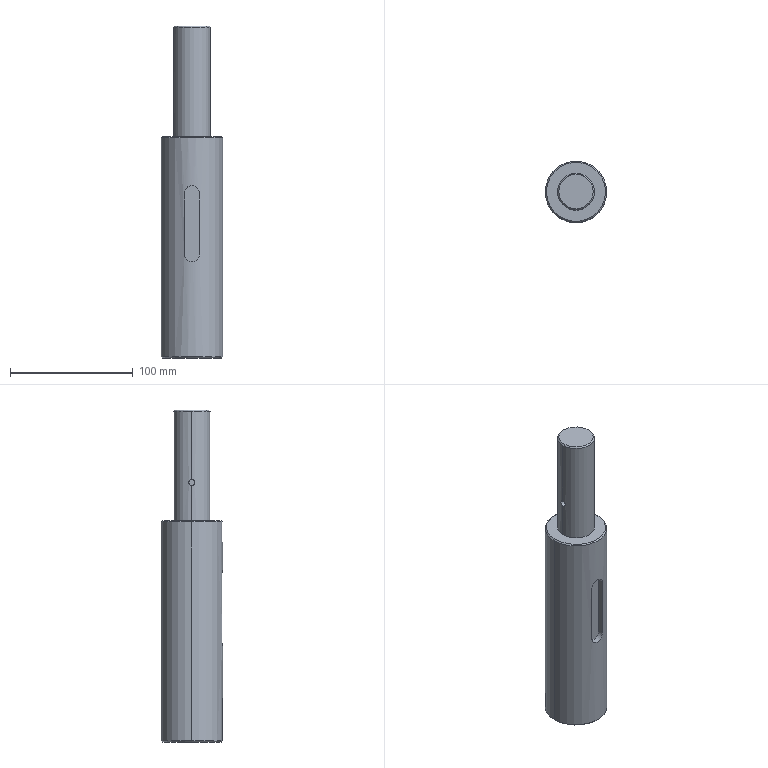Part | SolidWorks | features ICE 3, Chamfer 1, Extrusion 1 | 1 solid | 22 faces | box 50 x 50 x 270 mm | volume 413348 mm3 | cylinder 9 | plane 7 | cone 6 | commonest cylinder face diameters 12 x3 5 x2 30 x2 50 x2
STEP:
#1=CARTESIAN_POINT('',(-15.,0.,213.5));
#2=VERTEX_POINT('',#1);
#3=CARTESIAN_POINT('',(-15.,0.,208.5));
#4=VERTEX_POINT('',#3);
#5=CARTESIAN_POINT('',(-15.,0.,213.5));
#6=CARTESIAN_POINT('',(-15.,-0.1655,213.5));
#7=CARTESIAN_POINT('',(-14.997,-0.3282,213.484));
#8=CARTESIAN_POINT('',(-14.987,-0.6481,213.42));
#9=CARTESIAN_POINT('',(-14.979,-0.8071,213.372));
#10=CARTESIAN_POINT('',(-14.96,-1.11,213.246));
#11=CARTESIAN_POINT('',(-14.948,-1.253,213.169));
#12=CARTESIAN_POINT('',(-14.923,-1.525,212.988));
#13=CARTESIAN_POINT('',(-14.909,-1.653,212.882));
#14=CARTESIAN_POINT('',(-14.868,-1.998,212.537));
#15=CARTESIAN_POINT('',(-14.841,-2.184,212.259));
#16=CARTESIAN_POINT('',(-14.811,-2.372,211.808));
#17=CARTESIAN_POINT('',(-14.804,-2.42,211.65));
#18=CARTESIAN_POINT('',(-14.793,-2.484,211.327));
#19=CARTESIAN_POINT('',(-14.79,-2.5,211.164));
#20=CARTESIAN_POINT('',(-14.79,-2.5,210.838));
#21=CARTESIAN_POINT('',(-14.793,-2.484,210.672));
#22=CARTESIAN_POINT('',(-14.804,-2.42,210.351));
#23=CARTESIAN_POINT('',(-14.811,-2.372,210.195));
#24=CARTESIAN_POINT('',(-14.831,-2.247,209.892));
#25=CARTESIAN_POINT('',(-14.843,-2.169,209.746));
#26=CARTESIAN_POINT('',(-14.868,-1.988,209.475));
#27=CARTESIAN_POINT('',(-14.882,-1.884,209.349));
#28=CARTESIAN_POINT('',(-14.909,-1.651,209.116));
#29=CARTESIAN_POINT('',(-14.923,-1.525,209.013));
#30=CARTESIAN_POINT('',(-14.948,-1.255,208.832));
#31=CARTESIAN_POINT('',(-14.96,-1.109,208.753));
#32=CARTESIAN_POINT('',(-14.979,-0.8061,208.628));
#33=CARTESIAN_POINT('',(-14.987,-0.6502,208.58));
#34=CARTESIAN_POINT('',(-14.997,-0.3292,208.516));
#35=CARTESIAN_POINT('',(-15.,-0.1633,208.5));
#36=CARTESIAN_POINT('',(-15.,0.,208.5));
#37=B_SPLINE_CURVE_WITH_KNOTS('',3,(#5,#6,#7,#8,#9,#10,#11,#12,#13,#14,#15,#16,#17,#18,#19,#20,#21,#22,#23,#24,#25,#26,#27,#28,#29,#30,#31,#32,#33,#34,#35,#36),.UNSPECIFIED.,.F.,.F.,(4,2,2,2,2,2,2,2,2,2,2,2,2,2,2,4),(0.,0.0004894,0.0009787,0.001468,0.001957,0.002936,0.003426,0.003915,0.004404,0.004894,0.005383,0.005872,0.006362,0.006851,0.00734,0.00783),.UNSPECIFIED.);
#38=EDGE_CURVE('',#2,#4,#37,.T.);
#39=ORIENTED_EDGE('',*,*,#38,.F.);
#40=CARTESIAN_POINT('',(-10.,0.,213.5));
#41=VERTEX_POINT('',#40);
#42=CARTESIAN_POINT('',(-20.,0.,213.5));
#43=DIRECTION('',(1.,0.,0.));
#44=VECTOR('',#43,1000.);
#45=LINE('',#42,#44);
#46=EDGE_CURVE('',#2,#41,#45,.T.);
#47=ORIENTED_EDGE('',*,*,#46,.T.);
#48=CARTESIAN_POINT('',(-10.,0.,208.5));
#49=VERTEX_POINT('',#48);
#50=CARTESIAN_POINT('',(-10.,0.,211.));
#51=DIRECTION('',(1.,0.,0.));
#52=DIRECTION('',(0.,0.,-1.));
#53=AXIS2_PLACEMENT_3D('',#50,#51,#52);
#54=CIRCLE('',#53,2.5);
#55=EDGE_CURVE('',#41,#49,#54,.T.);
#56=ORIENTED_EDGE('',*,*,#55,.T.);
#57=CARTESIAN_POINT('',(-20.,0.,208.5));
#58=DIRECTION('',(1.,0.,0.));
#59=VECTOR('',#58,1000.);
#60=LINE('',#57,#59);
#61=EDGE_CURVE('',#4,#49,#60,.T.);
#62=ORIENTED_EDGE('',*,*,#61,.F.);
#63=EDGE_LOOP('',(#39,#47,#56,#62));
#64=FACE_OUTER_BOUND('',#63,.T.);
#65=CARTESIAN_POINT('',(-20.,0.,211.));
#66=DIRECTION('',(1.,0.,0.));
#67=DIRECTION('',(0.,0.,-1.));
#68=AXIS2_PLACEMENT_3D('',#65,#66,#67);
#69=CYLINDRICAL_SURFACE('',#68,2.5);
#70=ADVANCED_FACE('',(#64),#69,.F.);
#71=CARTESIAN_POINT('',(-24.,0.,0.));
#72=VERTEX_POINT('',#71);
#73=CARTESIAN_POINT('',(24.,0.,0.));
#74=VERTEX_POINT('',#73);
#75=CARTESIAN_POINT('',(0.,0.,0.));
#76=DIRECTION('',(0.,0.,-1.));
#77=DIRECTION('',(1.,0.,0.));
#78=AXIS2_PLACEMENT_3D('',#75,#76,#77);
#79=CIRCLE('',#78,24.);
#80=EDGE_CURVE('',#72,#74,#79,.T.);
#81=ORIENTED_EDGE('',*,*,#80,.F.);
#82=CARTESIAN_POINT('',(-25.,0.,1.));
#83=VERTEX_POINT('',#82);
#84=CARTESIAN_POINT('',(-25.,0.,1.));
#85=DIRECTION('',(-0.7071,0.,0.7071));
#86=VECTOR('',#85,1000.);
#87=LINE('',#84,#86);
#88=EDGE_CURVE('',#72,#83,#87,.T.);
#89=ORIENTED_EDGE('',*,*,#88,.T.);
#90=CARTESIAN_POINT('',(25.,0.,1.));
#91=VERTEX_POINT('',#90);
#92=CARTESIAN_POINT('',(0.,0.,1.));
#93=DIRECTION('',(0.,0.,1.));
#94=DIRECTION('',(1.,0.,0.));
#95=AXIS2_PLACEMENT_3D('',#92,#93,#94);
#96=CIRCLE('',#95,25.);
#97=EDGE_CURVE('',#91,#83,#96,.T.);
#98=ORIENTED_EDGE('',*,*,#97,.F.);
#99=CARTESIAN_POINT('',(25.,0.,1.));
#100=DIRECTION('',(0.7071,0.,0.7071));
#101=VECTOR('',#100,1000.);
#102=LINE('',#99,#101);
#103=EDGE_CURVE('',#74,#91,#102,.T.);
#104=ORIENTED_EDGE('',*,*,#103,.F.);
#105=EDGE_LOOP('',(#81,#89,#98,#104));
#106=FACE_OUTER_BOUND('',#105,.T.);
#107=CARTESIAN_POINT('',(0.,0.,1.));
#108=DIRECTION('',(0.,0.,1.));
#109=DIRECTION('',(1.,0.,0.));
#110=AXIS2_PLACEMENT_3D('',#107,#108,#109);
#111=CONICAL_SURFACE('',#110,25.,0.7854);
#112=ADVANCED_FACE('',(#106),#111,.T.);
#113=CARTESIAN_POINT('',(14.,0.,270.));
#114=VERTEX_POINT('',#113);
#115=CARTESIAN_POINT('',(-14.,0.,270.));
#116=VERTEX_POINT('',#115);
#117=CARTESIAN_POINT('',(0.,0.,270.));
#118=DIRECTION('',(0.,0.,1.));
#119=DIRECTION('',(1.,0.,0.));
#120=AXIS2_PLACEMENT_3D('',#117,#118,#119);
#121=CIRCLE('',#120,14.);
#122=EDGE_CURVE('',#114,#116,#121,.T.);
#123=ORIENTED_EDGE('',*,*,#122,.F.);
#124=CARTESIAN_POINT('',(15.,0.,269.));
#125=VERTEX_POINT('',#124);
#126=CARTESIAN_POINT('',(14.,0.,270.));
#127=DIRECTION('',(0.7071,0.,-0.7071));
#128=VECTOR('',#127,1000.);
#129=LINE('',#126,#128);
#130=EDGE_CURVE('',#114,#125,#129,.T.);
#131=ORIENTED_EDGE('',*,*,#130,.T.);
#132=CARTESIAN_POINT('',(-15.,0.,269.));
#133=VERTEX_POINT('',#132);
#134=CARTESIAN_POINT('',(0.,0.,269.));
#135=DIRECTION('',(0.,0.,-1.));
#136=DIRECTION('',(1.,0.,0.));
#137=AXIS2_PLACEMENT_3D('',#134,#135,#136);
#138=CIRCLE('',#137,15.);
#139=EDGE_CURVE('',#133,#125,#138,.T.);
#140=ORIENTED_EDGE('',*,*,#139,.F.);
#141=CARTESIAN_POINT('',(-14.,0.,270.));
#142=DIRECTION('',(-0.7071,0.,-0.7071));
#143=VECTOR('',#142,1000.);
#144=LINE('',#141,#143);
#145=EDGE_CURVE('',#116,#133,#144,.T.);
#146=ORIENTED_EDGE('',*,*,#145,.F.);
#147=EDGE_LOOP('',(#123,#131,#140,#146));
#148=FACE_OUTER_BOUND('',#147,.T.);
#149=CARTESIAN_POINT('',(0.,0.,270.));
#150=DIRECTION('',(0.,0.,-1.));
#151=DIRECTION('',(-1.,0.,0.));
#152=AXIS2_PLACEMENT_3D('',#149,#150,#151);
#153=CONICAL_SURFACE('',#152,14.,0.7854);
#154=ADVANCED_FACE('',(#148),#153,.T.);
#155=CARTESIAN_POINT('',(24.,0.,180.));
#156=VERTEX_POINT('',#155);
#157=CARTESIAN_POINT('',(-24.,0.,180.));
#158=VERTEX_POINT('',#157);
#159=CARTESIAN_POINT('',(0.,0.,180.));
#160=DIRECTION('',(0.,0.,1.));
#161=DIRECTION('',(1.,0.,0.));
#162=AXIS2_PLACEMENT_3D('',#159,#160,#161);
#163=CIRCLE('',#162,24.);
#164=EDGE_CURVE('',#156,#158,#163,.T.);
#165=ORIENTED_EDGE('',*,*,#164,.F.);
#166=CARTESIAN_POINT('',(25.,0.,179.));
#167=VERTEX_POINT('',#166);
#168=CARTESIAN_POINT('',(24.,0.,180.));
#169=DIRECTION('',(0.7071,0.,-0.7071));
#170=VECTOR('',#169,1000.);
#171=LINE('',#168,#170);
#172=EDGE_CURVE('',#156,#167,#171,.T.);
#173=ORIENTED_EDGE('',*,*,#172,.T.);
#174=CARTESIAN_POINT('',(-25.,0.,179.));
#175=VERTEX_POINT('',#174);
#176=CARTESIAN_POINT('',(0.,0.,179.));
#177=DIRECTION('',(0.,0.,-1.));
#178=DIRECTION('',(1.,0.,0.));
#179=AXIS2_PLACEMENT_3D('',#176,#177,#178);
#180=CIRCLE('',#179,25.);
#181=EDGE_CURVE('',#175,#167,#180,.T.);
#182=ORIENTED_EDGE('',*,*,#181,.F.);
#183=CARTESIAN_POINT('',(-24.,0.,180.));
#184=DIRECTION('',(-0.7071,0.,-0.7071));
#185=VECTOR('',#184,1000.);
#186=LINE('',#183,#185);
#187=EDGE_CURVE('',#158,#175,#186,.T.);
#188=ORIENTED_EDGE('',*,*,#187,.F.);
#189=EDGE_LOOP('',(#165,#173,#182,#188));
#190=FACE_OUTER_BOUND('',#189,.T.);
#191=CARTESIAN_POINT('',(0.,0.,180.));
#192=DIRECTION('',(0.,0.,-1.));
#193=DIRECTION('',(-1.,0.,0.));
#194=AXIS2_PLACEMENT_3D('',#191,#192,#193);
#195=CONICAL_SURFACE('',#194,24.,0.7854);
#196=ADVANCED_FACE('',(#190),#195,.T.);
#197=CARTESIAN_POINT('',(0.,-25.,140.23));
#198=VERTEX_POINT('',#197);
#199=CARTESIAN_POINT('',(6.,-24.269,134.23));
#200=VERTEX_POINT('',#199);
#201=CARTESIAN_POINT('',(0.,-25.,140.23));
#202=CARTESIAN_POINT('',(0.3927,-25.,140.23));
#203=CARTESIAN_POINT('',(0.7916,-24.99,140.19));
#204=CARTESIAN_POINT('',(1.562,-24.954,140.036));
#205=CARTESIAN_POINT('',(1.936,-24.928,139.923));
#206=CARTESIAN_POINT('',(2.482,-24.877,139.696));
#207=CARTESIAN_POINT('',(2.661,-24.859,139.611));
#208=CARTESIAN_POINT('',(3.007,-24.819,139.426));
#209=CARTESIAN_POINT('',(3.174,-24.798,139.325));
#210=CARTESIAN_POINT('',(3.498,-24.755,139.108));
#211=CARTESIAN_POINT('',(3.655,-24.732,138.992));
#212=CARTESIAN_POINT('',(3.957,-24.685,138.744));
#213=CARTESIAN_POINT('',(4.104,-24.661,138.612));
#214=CARTESIAN_POINT('',(4.521,-24.59,138.195));
#215=CARTESIAN_POINT('',(4.768,-24.542,137.894));
#216=CARTESIAN_POINT('',(5.202,-24.454,137.246));
#217=CARTESIAN_POINT('',(5.39,-24.413,136.895));
#218=CARTESIAN_POINT('',(5.691,-24.344,136.171));
#219=CARTESIAN_POINT('',(5.805,-24.317,135.797));
#220=CARTESIAN_POINT('',(5.96,-24.279,135.026));
#221=CARTESIAN_POINT('',(6.,-24.269,134.628));
#222=CARTESIAN_POINT('',(6.,-24.269,134.23));
#223=B_SPLINE_CURVE_WITH_KNOTS('',3,(#201,#202,#203,#204,#205,#206,#207,#208,#209,#210,#211,#212,#213,#214,#215,#216,#217,#218,#219,#220,#221,#222),.UNSPECIFIED.,.F.,.F.,(4,2,2,2,2,2,2,2,2,2,4),(0.009416,0.01059,0.01177,0.01236,0.01294,0.01353,0.01412,0.01529,0.01647,0.01765,0.01882),.UNSPECIFIED.);
#224=EDGE_CURVE('',#198,#200,#223,.T.);
#225=ORIENTED_EDGE('',*,*,#224,.F.);
#226=CARTESIAN_POINT('',(0.,-20.,140.23));
#227=VERTEX_POINT('',#226);
#228=CARTESIAN_POINT('',(0.,-140.,140.23));
#229=DIRECTION('',(0.,1.,0.));
#230=VECTOR('',#229,1000.);
#231=LINE('',#228,#230);
#232=EDGE_CURVE('',#198,#227,#231,.T.);
#233=ORIENTED_EDGE('',*,*,#232,.T.);
#234=CARTESIAN_POINT('',(6.,-20.,134.23));
#235=VERTEX_POINT('',#234);
#236=CARTESIAN_POINT('',(0.,-20.,134.23));
#237=DIRECTION('',(0.,1.,0.));
#238=DIRECTION('',(0.,0.,1.));
#239=AXIS2_PLACEMENT_3D('',#236,#237,#238);
#240=CIRCLE('',#239,6.);
#241=EDGE_CURVE('',#227,#235,#240,.T.);
#242=ORIENTED_EDGE('',*,*,#241,.T.);
#243=CARTESIAN_POINT('',(6.,-140.,134.23));
#244=DIRECTION('',(0.,1.,0.));
#245=VECTOR('',#244,1000.);
#246=LINE('',#243,#245);
#247=EDGE_CURVE('',#200,#235,#246,.T.);
#248=ORIENTED_EDGE('',*,*,#247,.F.);
#249=EDGE_LOOP('',(#225,#233,#242,#248));
#250=FACE_OUTER_BOUND('',#249,.T.);
#251=CARTESIAN_POINT('',(0.,-140.,134.23));
#252=DIRECTION('',(0.,1.,0.));
#253=DIRECTION('',(0.,0.,1.));
#254=AXIS2_PLACEMENT_3D('',#251,#252,#253);
#255=CYLINDRICAL_SURFACE('',#254,6.);
#256=ADVANCED_FACE('',(#250),#255,.F.);
#257=ORIENTED_EDGE('',*,*,#139,.T.);
#258=CARTESIAN_POINT('',(15.,0.,180.));
#259=VERTEX_POINT('',#258);
#260=CARTESIAN_POINT('',(15.,0.,270.));
#261=DIRECTION('',(0.,0.,-1.));
#262=VECTOR('',#261,1000.);
#263=LINE('',#260,#262);
#264=EDGE_CURVE('',#125,#259,#263,.T.);
#265=ORIENTED_EDGE('',*,*,#264,.T.);
#266=CARTESIAN_POINT('',(-15.,0.,180.));
#267=VERTEX_POINT('',#266);
#268=CARTESIAN_POINT('',(0.,0.,180.));
#269=DIRECTION('',(0.,0.,1.));
#270=DIRECTION('',(1.,0.,0.));
#271=AXIS2_PLACEMENT_3D('',#268,#269,#270);
#272=CIRCLE('',#271,15.);
#273=EDGE_CURVE('',#259,#267,#272,.T.);
#274=ORIENTED_EDGE('',*,*,#273,.T.);
#275=CARTESIAN_POINT('',(-15.,0.,270.));
#276=DIRECTION('',(0.,0.,-1.));
#277=VECTOR('',#276,1000.);
#278=LINE('',#275,#277);
#279=EDGE_CURVE('',#4,#267,#278,.T.);
#280=ORIENTED_EDGE('',*,*,#279,.F.);
#281=CARTESIAN_POINT('',(-15.,0.,208.5));
#282=CARTESIAN_POINT('',(-15.,0.3265,208.5));
#283=CARTESIAN_POINT('',(-14.989,0.656,208.566));
#284=CARTESIAN_POINT('',(-14.96,1.107,208.753));
#285=CARTESIAN_POINT('',(-14.948,1.253,208.831));
#286=CARTESIAN_POINT('',(-14.923,1.526,209.013));
#287=CARTESIAN_POINT('',(-14.909,1.651,209.116));
#288=CARTESIAN_POINT('',(-14.882,1.882,209.346));
#289=CARTESIAN_POINT('',(-14.868,1.987,209.475));
#290=CARTESIAN_POINT('',(-14.843,2.169,209.746));
#291=CARTESIAN_POINT('',(-14.831,2.246,209.889));
#292=CARTESIAN_POINT('',(-14.811,2.371,210.192));
#293=CARTESIAN_POINT('',(-14.804,2.42,210.35));
#294=CARTESIAN_POINT('',(-14.793,2.483,210.67));
#295=CARTESIAN_POINT('',(-14.79,2.5,210.833));
#296=CARTESIAN_POINT('',(-14.79,2.5,211.164));
#297=CARTESIAN_POINT('',(-14.793,2.484,211.326));
#298=CARTESIAN_POINT('',(-14.803,2.421,211.646));
#299=CARTESIAN_POINT('',(-14.811,2.372,211.805));
#300=CARTESIAN_POINT('',(-14.831,2.247,212.108));
#301=CARTESIAN_POINT('',(-14.842,2.17,212.251));
#302=CARTESIAN_POINT('',(-14.868,1.989,212.523));
#303=CARTESIAN_POINT('',(-14.882,1.884,212.651));
#304=CARTESIAN_POINT('',(-14.923,1.539,212.997));
#305=CARTESIAN_POINT('',(-14.95,1.261,213.183));
#306=CARTESIAN_POINT('',(-14.979,0.8099,213.371));
#307=CARTESIAN_POINT('',(-14.987,0.6518,213.419));
#308=CARTESIAN_POINT('',(-14.997,0.3289,213.484));
#309=CARTESIAN_POINT('',(-15.,0.1655,213.5));
#310=CARTESIAN_POINT('',(-15.,0.,213.5));
#311=B_SPLINE_CURVE_WITH_KNOTS('',3,(#281,#282,#283,#284,#285,#286,#287,#288,#289,#290,#291,#292,#293,#294,#295,#296,#297,#298,#299,#300,#301,#302,#303,#304,#305,#306,#307,#308,#309,#310),.UNSPECIFIED.,.F.,.F.,(4,2,2,2,2,2,2,2,2,2,2,2,2,2,4),(0.00783,0.008808,0.009298,0.009787,0.01028,0.01077,0.01125,0.01174,0.01223,0.01272,0.01321,0.0137,0.01468,0.01517,0.01566),.UNSPECIFIED.);
#312=EDGE_CURVE('',#4,#2,#311,.T.);
#313=ORIENTED_EDGE('',*,*,#312,.T.);
#314=CARTESIAN_POINT('',(-15.,0.,270.));
#315=DIRECTION('',(0.,0.,-1.));
#316=VECTOR('',#315,1000.);
#317=LINE('',#314,#316);
#318=EDGE_CURVE('',#133,#2,#317,.T.);
#319=ORIENTED_EDGE('',*,*,#318,.F.);
#320=EDGE_LOOP('',(#257,#265,#274,#280,#313,#319));
#321=FACE_OUTER_BOUND('',#320,.T.);
#322=CARTESIAN_POINT('',(0.,0.,270.));
#323=DIRECTION('',(0.,0.,-1.));
#324=DIRECTION('',(-1.,0.,0.));
#325=AXIS2_PLACEMENT_3D('',#322,#323,#324);
#326=CYLINDRICAL_SURFACE('',#325,15.);
#327=ADVANCED_FACE('',(#321),#326,.T.);
#328=ORIENTED_EDGE('',*,*,#181,.T.);
#329=CARTESIAN_POINT('',(25.,0.,180.));
#330=DIRECTION('',(0.,0.,-1.));
#331=VECTOR('',#330,1000.);
#332=LINE('',#329,#331);
#333=EDGE_CURVE('',#167,#91,#332,.T.);
#334=ORIENTED_EDGE('',*,*,#333,.T.);
#335=ORIENTED_EDGE('',*,*,#97,.T.);
#336=CARTESIAN_POINT('',(-25.,0.,180.));
#337=DIRECTION('',(0.,0.,-1.));
#338=VECTOR('',#337,1000.);
#339=LINE('',#336,#338);
#340=EDGE_CURVE('',#175,#83,#339,.T.);
#341=ORIENTED_EDGE('',*,*,#340,.F.);
#342=EDGE_LOOP('',(#328,#334,#335,#341));
#343=FACE_OUTER_BOUND('',#342,.T.);
#344=CARTESIAN_POINT('',(0.,0.,180.));
#345=DIRECTION('',(0.,0.,-1.));
#346=DIRECTION('',(-1.,0.,0.));
#347=AXIS2_PLACEMENT_3D('',#344,#345,#346);
#348=CYLINDRICAL_SURFACE('',#347,25.);
#349=ADVANCED_FACE('',(#343),#348,.T.);
#350=ORIENTED_EDGE('',*,*,#333,.F.);
#351=CARTESIAN_POINT('',(0.,0.,179.));
#352=DIRECTION('',(0.,0.,-1.));
#353=DIRECTION('',(1.,0.,0.));
#354=AXIS2_PLACEMENT_3D('',#351,#352,#353);
#355=CIRCLE('',#354,25.);
#356=EDGE_CURVE('',#167,#175,#355,.T.);
#357=ORIENTED_EDGE('',*,*,#356,.T.);
#358=ORIENTED_EDGE('',*,*,#340,.T.);
#359=CARTESIAN_POINT('',(0.,0.,1.));
#360=DIRECTION('',(0.,0.,1.));
#361=DIRECTION('',(1.,0.,0.));
#362=AXIS2_PLACEMENT_3D('',#359,#360,#361);
#363=CIRCLE('',#362,25.);
#364=EDGE_CURVE('',#83,#91,#363,.T.);
#365=ORIENTED_EDGE('',*,*,#364,.T.);
#366=EDGE_LOOP('',(#350,#357,#358,#365));
#367=FACE_OUTER_BOUND('',#366,.T.);
#368=CARTESIAN_POINT('',(6.,-24.269,84.23));
#369=VERTEX_POINT('',#368);
#370=CARTESIAN_POINT('',(6.,-24.269,180.));
#371=DIRECTION('',(0.,0.,-1.));
#372=VECTOR('',#371,1000.);
#373=LINE('',#370,#372);
#374=EDGE_CURVE('',#200,#369,#373,.T.);
#375=ORIENTED_EDGE('',*,*,#374,.T.);
#376=CARTESIAN_POINT('',(-6.,-24.269,84.23));
#377=VERTEX_POINT('',#376);
#378=CARTESIAN_POINT('',(6.,-24.269,84.23));
#379=CARTESIAN_POINT('',(6.,-24.269,83.832));
#380=CARTESIAN_POINT('',(5.961,-24.279,83.441));
#381=CARTESIAN_POINT('',(5.846,-24.307,82.865));
#382=CARTESIAN_POINT('',(5.798,-24.318,82.674));
#383=CARTESIAN_POINT('',(5.683,-24.345,82.297));
#384=CARTESIAN_POINT('',(5.616,-24.361,82.109));
#385=CARTESIAN_POINT('',(5.39,-24.413,81.565));
#386=CARTESIAN_POINT('',(5.206,-24.453,81.221));
#387=CARTESIAN_POINT('',(4.771,-24.542,80.57));
#388=CARTESIAN_POINT('',(4.518,-24.59,80.263));
#389=CARTESIAN_POINT('',(3.967,-24.685,79.712));
#390=CARTESIAN_POINT('',(3.666,-24.732,79.464));
#391=CARTESIAN_POINT('',(3.011,-24.82,79.025));
#392=CARTESIAN_POINT('',(2.664,-24.86,78.84));
#393=CARTESIAN_POINT('',(2.123,-24.91,78.615));
#394=CARTESIAN_POINT('',(1.939,-24.925,78.548));
#395=CARTESIAN_POINT('',(1.563,-24.952,78.434));
#396=CARTESIAN_POINT('',(1.37,-24.963,78.385));
#397=CARTESIAN_POINT('',(0.7883,-24.991,78.269));
#398=CARTESIAN_POINT('',(0.3981,-25.,78.23));
#399=CARTESIAN_POINT('',(-0.3876,-25.,78.23));
#400=CARTESIAN_POINT('',(-0.7868,-24.991,78.269));
#401=CARTESIAN_POINT('',(-1.557,-24.954,78.422));
#402=CARTESIAN_POINT('',(-1.932,-24.928,78.536));
#403=CARTESIAN_POINT('',(-2.478,-24.878,78.762));
#404=CARTESIAN_POINT('',(-2.658,-24.859,78.847));
#405=CARTESIAN_POINT('',(-3.004,-24.819,79.032));
#406=CARTESIAN_POINT('',(-3.172,-24.799,79.133));
#407=CARTESIAN_POINT('',(-3.658,-24.733,79.458));
#408=CARTESIAN_POINT('',(-3.963,-24.686,79.707));
#409=CARTESIAN_POINT('',(-4.519,-24.59,80.263));
#410=CARTESIAN_POINT('',(-4.766,-24.542,80.565));
#411=CARTESIAN_POINT('',(-5.201,-24.454,81.213));
#412=CARTESIAN_POINT('',(-5.389,-24.413,81.564));
#413=CARTESIAN_POINT('',(-5.691,-24.344,82.288));
#414=CARTESIAN_POINT('',(-5.805,-24.317,82.662));
#415=CARTESIAN_POINT('',(-5.96,-24.279,83.434));
#416=CARTESIAN_POINT('',(-6.,-24.269,83.832));
#417=CARTESIAN_POINT('',(-6.,-24.269,84.23));
#418=B_SPLINE_CURVE_WITH_KNOTS('',3,(#378,#379,#380,#381,#382,#383,#384,#385,#386,#387,#388,#389,#390,#391,#392,#393,#394,#395,#396,#397,#398,#399,#400,#401,#402,#403,#404,#405,#406,#407,#408,#409,#410,#411,#412,#413,#414,#415,#416,#417),.UNSPECIFIED.,.F.,.F.,(4,2,2,2,2,2,2,2,2,2,2,2,2,2,2,2,2,2,2,4),(0.,0.001176,0.001765,0.002353,0.003529,0.004705,0.005882,0.007058,0.007646,0.008235,0.009411,0.01059,0.01176,0.01235,0.01294,0.01412,0.01529,0.01647,0.01765,0.01882),.UNSPECIFIED.);
#419=EDGE_CURVE('',#369,#377,#418,.T.);
#420=ORIENTED_EDGE('',*,*,#419,.T.);
#421=CARTESIAN_POINT('',(-6.,-24.269,134.23));
#422=VERTEX_POINT('',#421);
#423=CARTESIAN_POINT('',(-6.,-24.269,180.));
#424=DIRECTION('',(0.,0.,1.));
#425=VECTOR('',#424,1000.);
#426=LINE('',#423,#425);
#427=EDGE_CURVE('',#377,#422,#426,.T.);
#428=ORIENTED_EDGE('',*,*,#427,.T.);
#429=CARTESIAN_POINT('',(-6.,-24.269,134.23));
#430=CARTESIAN_POINT('',(-6.,-24.269,134.628));
#431=CARTESIAN_POINT('',(-5.961,-24.279,135.019));
#432=CARTESIAN_POINT('',(-5.846,-24.307,135.596));
#433=CARTESIAN_POINT('',(-5.798,-24.318,135.787));
#434=CARTESIAN_POINT('',(-5.683,-24.346,136.164));
#435=CARTESIAN_POINT('',(-5.616,-24.361,136.352));
#436=CARTESIAN_POINT('',(-5.389,-24.413,136.896));
#437=CARTESIAN_POINT('',(-5.205,-24.453,137.24));
#438=CARTESIAN_POINT('',(-4.769,-24.542,137.892));
#439=CARTESIAN_POINT('',(-4.517,-24.59,138.199));
#440=CARTESIAN_POINT('',(-3.965,-24.685,138.75));
#441=CARTESIAN_POINT('',(-3.664,-24.732,138.998));
#442=CARTESIAN_POINT('',(-3.008,-24.821,139.437));
#443=CARTESIAN_POINT('',(-2.661,-24.861,139.622));
#444=CARTESIAN_POINT('',(-2.119,-24.911,139.847));
#445=CARTESIAN_POINT('',(-1.935,-24.926,139.913));
#446=CARTESIAN_POINT('',(-1.559,-24.952,140.027));
#447=CARTESIAN_POINT('',(-1.365,-24.963,140.076));
#448=CARTESIAN_POINT('',(-0.7835,-24.991,140.192));
#449=CARTESIAN_POINT('',(-0.3931,-25.,140.23));
#450=CARTESIAN_POINT('',(0.,-25.,140.23));
#451=B_SPLINE_CURVE_WITH_KNOTS('',3,(#429,#430,#431,#432,#433,#434,#435,#436,#437,#438,#439,#440,#441,#442,#443,#444,#445,#446,#447,#448,#449,#450),.UNSPECIFIED.,.F.,.F.,(4,2,2,2,2,2,2,2,2,2,4),(0.,0.001177,0.001766,0.002354,0.003531,0.004708,0.005885,0.007062,0.007651,0.008239,0.009416),.UNSPECIFIED.);
#452=EDGE_CURVE('',#422,#198,#451,.T.);
#453=ORIENTED_EDGE('',*,*,#452,.T.);
#454=ORIENTED_EDGE('',*,*,#224,.T.);
#455=EDGE_LOOP('',(#375,#420,#428,#453,#454));
#456=FACE_BOUND('',#455,.T.);
#457=CARTESIAN_POINT('',(0.,0.,180.));
#458=DIRECTION('',(0.,0.,-1.));
#459=DIRECTION('',(-1.,0.,0.));
#460=AXIS2_PLACEMENT_3D('',#457,#458,#459);
#461=CYLINDRICAL_SURFACE('',#460,25.);
#462=ADVANCED_FACE('',(#367,#456),#461,.T.);
#463=CARTESIAN_POINT('',(0.,0.,180.));
#464=DIRECTION('',(0.,0.,1.));
#465=DIRECTION('',(1.,0.,0.));
#466=AXIS2_PLACEMENT_3D('',#463,#464,#465);
#467=CIRCLE('',#466,24.);
#468=EDGE_CURVE('',#158,#156,#467,.T.);
#469=ORIENTED_EDGE('',*,*,#468,.T.);
#470=ORIENTED_EDGE('',*,*,#164,.T.);
#471=EDGE_LOOP('',(#469,#470));
#472=FACE_OUTER_BOUND('',#471,.T.);
#473=CARTESIAN_POINT('',(0.,0.,180.));
#474=DIRECTION('',(0.,0.,1.));
#475=DIRECTION('',(1.,0.,0.));
#476=AXIS2_PLACEMENT_3D('',#473,#474,#475);
#477=CIRCLE('',#476,15.);
#478=EDGE_CURVE('',#267,#259,#477,.T.);
#479=ORIENTED_EDGE('',*,*,#478,.F.);
#480=ORIENTED_EDGE('',*,*,#273,.F.);
#481=EDGE_LOOP('',(#479,#480));
#482=FACE_BOUND('',#481,.T.);
#483=CARTESIAN_POINT('',(0.,0.,180.));
#484=DIRECTION('',(0.,0.,1.));
#485=DIRECTION('',(1.,0.,0.));
#486=AXIS2_PLACEMENT_3D('',#483,#484,#485);
#487=PLANE('',#486);
#488=ADVANCED_FACE('',(#472,#482),#487,.T.);
#489=CARTESIAN_POINT('',(0.,0.,0.));
#490=DIRECTION('',(0.,0.,-1.));
#491=DIRECTION('',(1.,0.,0.));
#492=AXIS2_PLACEMENT_3D('',#489,#490,#491);
#493=CIRCLE('',#492,24.);
#494=EDGE_CURVE('',#74,#72,#493,.T.);
#495=ORIENTED_EDGE('',*,*,#494,.T.);
#496=ORIENTED_EDGE('',*,*,#80,.T.);
#497=EDGE_LOOP('',(#495,#496));
#498=FACE_OUTER_BOUND('',#497,.T.);
#499=CARTESIAN_POINT('',(0.,0.,0.));
#500=DIRECTION('',(0.,0.,1.));
#501=DIRECTION('',(1.,0.,0.));
#502=AXIS2_PLACEMENT_3D('',#499,#500,#501);
#503=PLANE('',#502);
#504=ADVANCED_FACE('',(#498),#503,.F.);
#505=ORIENTED_EDGE('',*,*,#264,.F.);
#506=CARTESIAN_POINT('',(0.,0.,269.));
#507=DIRECTION('',(0.,0.,-1.));
#508=DIRECTION('',(1.,0.,0.));
#509=AXIS2_PLACEMENT_3D('',#506,#507,#508);
#510=CIRCLE('',#509,15.);
#511=EDGE_CURVE('',#125,#133,#510,.T.);
#512=ORIENTED_EDGE('',*,*,#511,.T.);
#513=ORIENTED_EDGE('',*,*,#318,.T.);
#514=ORIENTED_EDGE('',*,*,#38,.T.);
#515=ORIENTED_EDGE('',*,*,#279,.T.);
#516=ORIENTED_EDGE('',*,*,#478,.T.);
#517=EDGE_LOOP('',(#505,#512,#513,#514,#515,#516));
#518=FACE_OUTER_BOUND('',#517,.T.);
#519=CARTESIAN_POINT('',(0.,0.,270.));
#520=DIRECTION('',(0.,0.,-1.));
#521=DIRECTION('',(-1.,0.,0.));
#522=AXIS2_PLACEMENT_3D('',#519,#520,#521);
#523=CYLINDRICAL_SURFACE('',#522,15.);
#524=ADVANCED_FACE('',(#518),#523,.T.);
#525=CARTESIAN_POINT('',(0.,0.,270.));
#526=DIRECTION('',(0.,0.,1.));
#527=DIRECTION('',(1.,0.,0.));
#528=AXIS2_PLACEMENT_3D('',#525,#526,#527);
#529=CIRCLE('',#528,14.);
#530=EDGE_CURVE('',#116,#114,#529,.T.);
#531=ORIENTED_EDGE('',*,*,#530,.T.);
#532=ORIENTED_EDGE('',*,*,#122,.T.);
#533=EDGE_LOOP('',(#531,#532));
#534=FACE_OUTER_BOUND('',#533,.T.);
#535=CARTESIAN_POINT('',(0.,0.,270.));
#536=DIRECTION('',(0.,0.,1.));
#537=DIRECTION('',(1.,0.,0.));
#538=AXIS2_PLACEMENT_3D('',#535,#536,#537);
#539=PLANE('',#538);
#540=ADVANCED_FACE('',(#534),#539,.T.);
#541=CARTESIAN_POINT('',(6.,-20.,84.23));
#542=VERTEX_POINT('',#541);
#543=CARTESIAN_POINT('',(6.,-140.,84.23));
#544=DIRECTION('',(0.,1.,0.));
#545=VECTOR('',#544,1000.);
#546=LINE('',#543,#545);
#547=EDGE_CURVE('',#369,#542,#546,.T.);
#548=ORIENTED_EDGE('',*,*,#547,.T.);
#549=CARTESIAN_POINT('',(-6.,-20.,84.23));
#550=VERTEX_POINT('',#549);
#551=CARTESIAN_POINT('',(0.,-20.,84.23));
#552=DIRECTION('',(0.,1.,0.));
#553=DIRECTION('',(0.,0.,1.));
#554=AXIS2_PLACEMENT_3D('',#551,#552,#553);
#555=CIRCLE('',#554,6.);
#556=EDGE_CURVE('',#542,#550,#555,.T.);
#557=ORIENTED_EDGE('',*,*,#556,.T.);
#558=CARTESIAN_POINT('',(-6.,-140.,84.23));
#559=DIRECTION('',(0.,1.,0.));
#560=VECTOR('',#559,1000.);
#561=LINE('',#558,#560);
#562=EDGE_CURVE('',#377,#550,#561,.T.);
#563=ORIENTED_EDGE('',*,*,#562,.F.);
#564=ORIENTED_EDGE('',*,*,#419,.F.);
#565=EDGE_LOOP('',(#548,#557,#563,#564));
#566=FACE_OUTER_BOUND('',#565,.T.);
#567=CARTESIAN_POINT('',(0.,-140.,84.23));
#568=DIRECTION('',(0.,1.,0.));
#569=DIRECTION('',(0.,0.,1.));
#570=AXIS2_PLACEMENT_3D('',#567,#568,#569);
#571=CYLINDRICAL_SURFACE('',#570,6.);
#572=ADVANCED_FACE('',(#566),#571,.F.);
#573=ORIENTED_EDGE('',*,*,#247,.T.);
#574=CARTESIAN_POINT('',(6.,-20.,84.23));
#575=DIRECTION('',(0.,0.,-1.));
#576=VECTOR('',#575,1000.);
#577=LINE('',#574,#576);
#578=EDGE_CURVE('',#235,#542,#577,.T.);
#579=ORIENTED_EDGE('',*,*,#578,.T.);
#580=ORIENTED_EDGE('',*,*,#547,.F.);
#581=ORIENTED_EDGE('',*,*,#374,.F.);
#582=EDGE_LOOP('',(#573,#579,#580,#581));
#583=FACE_OUTER_BOUND('',#582,.T.);
#584=CARTESIAN_POINT('',(6.,-140.,84.23));
#585=DIRECTION('',(1.,0.,0.));
#586=DIRECTION('',(0.,0.,-1.));
#587=AXIS2_PLACEMENT_3D('',#584,#585,#586);
#588=PLANE('',#587);
#589=ADVANCED_FACE('',(#583),#588,.F.);
#590=ORIENTED_EDGE('',*,*,#232,.F.);
#591=ORIENTED_EDGE('',*,*,#452,.F.);
#592=CARTESIAN_POINT('',(-6.,-20.,134.23));
#593=VERTEX_POINT('',#592);
#594=CARTESIAN_POINT('',(-6.,-140.,134.23));
#595=DIRECTION('',(0.,1.,0.));
#596=VECTOR('',#595,1000.);
#597=LINE('',#594,#596);
#598=EDGE_CURVE('',#422,#593,#597,.T.);
#599=ORIENTED_EDGE('',*,*,#598,.T.);
#600=CARTESIAN_POINT('',(0.,-20.,134.23));
#601=DIRECTION('',(0.,1.,0.));
#602=DIRECTION('',(0.,0.,1.));
#603=AXIS2_PLACEMENT_3D('',#600,#601,#602);
#604=CIRCLE('',#603,6.);
#605=EDGE_CURVE('',#593,#227,#604,.T.);
#606=ORIENTED_EDGE('',*,*,#605,.T.);
#607=EDGE_LOOP('',(#590,#591,#599,#606));
#608=FACE_OUTER_BOUND('',#607,.T.);
#609=CARTESIAN_POINT('',(0.,-140.,134.23));
#610=DIRECTION('',(0.,1.,0.));
#611=DIRECTION('',(0.,0.,1.));
#612=AXIS2_PLACEMENT_3D('',#609,#610,#611);
#613=CYLINDRICAL_SURFACE('',#612,6.);
#614=ADVANCED_FACE('',(#608),#613,.F.);
#615=ORIENTED_EDGE('',*,*,#562,.T.);
#616=CARTESIAN_POINT('',(-6.,-20.,84.23));
#617=DIRECTION('',(0.,0.,1.));
#618=VECTOR('',#617,1000.);
#619=LINE('',#616,#618);
#620=EDGE_CURVE('',#550,#593,#619,.T.);
#621=ORIENTED_EDGE('',*,*,#620,.T.);
#622=ORIENTED_EDGE('',*,*,#598,.F.);
#623=ORIENTED_EDGE('',*,*,#427,.F.);
#624=EDGE_LOOP('',(#615,#621,#622,#623));
#625=FACE_OUTER_BOUND('',#624,.T.);
#626=CARTESIAN_POINT('',(-6.,-140.,84.23));
#627=DIRECTION('',(-1.,0.,0.));
#628=DIRECTION('',(0.,0.,1.));
#629=AXIS2_PLACEMENT_3D('',#626,#627,#628);
#630=PLANE('',#629);
#631=ADVANCED_FACE('',(#625),#630,.F.);
#632=ORIENTED_EDGE('',*,*,#556,.F.);
#633=ORIENTED_EDGE('',*,*,#578,.F.);
#634=ORIENTED_EDGE('',*,*,#241,.F.);
#635=ORIENTED_EDGE('',*,*,#605,.F.);
#636=ORIENTED_EDGE('',*,*,#620,.F.);
#637=EDGE_LOOP('',(#632,#633,#634,#635,#636));
#638=FACE_OUTER_BOUND('',#637,.T.);
#639=CARTESIAN_POINT('',(0.,-20.,84.23));
#640=DIRECTION('',(0.,1.,0.));
#641=DIRECTION('',(0.,0.,1.));
#642=AXIS2_PLACEMENT_3D('',#639,#640,#641);
#643=PLANE('',#642);
#644=ADVANCED_FACE('',(#638),#643,.F.);
#645=ORIENTED_EDGE('',*,*,#172,.F.);
#646=ORIENTED_EDGE('',*,*,#468,.F.);
#647=ORIENTED_EDGE('',*,*,#187,.T.);
#648=ORIENTED_EDGE('',*,*,#356,.F.);
#649=EDGE_LOOP('',(#645,#646,#647,#648));
#650=FACE_OUTER_BOUND('',#649,.T.);
#651=CARTESIAN_POINT('',(0.,0.,180.));
#652=DIRECTION('',(0.,0.,-1.));
#653=DIRECTION('',(-1.,0.,0.));
#654=AXIS2_PLACEMENT_3D('',#651,#652,#653);
#655=CONICAL_SURFACE('',#654,24.,0.7854);
#656=ADVANCED_FACE('',(#650),#655,.T.);
#657=ORIENTED_EDGE('',*,*,#130,.F.);
#658=ORIENTED_EDGE('',*,*,#530,.F.);
#659=ORIENTED_EDGE('',*,*,#145,.T.);
#660=ORIENTED_EDGE('',*,*,#511,.F.);
#661=EDGE_LOOP('',(#657,#658,#659,#660));
#662=FACE_OUTER_BOUND('',#661,.T.);
#663=CARTESIAN_POINT('',(0.,0.,270.));
#664=DIRECTION('',(0.,0.,-1.));
#665=DIRECTION('',(-1.,0.,0.));
#666=AXIS2_PLACEMENT_3D('',#663,#664,#665);
#667=CONICAL_SURFACE('',#666,14.,0.7854);
#668=ADVANCED_FACE('',(#662),#667,.T.);
#669=ORIENTED_EDGE('',*,*,#88,.F.);
#670=ORIENTED_EDGE('',*,*,#494,.F.);
#671=ORIENTED_EDGE('',*,*,#103,.T.);
#672=ORIENTED_EDGE('',*,*,#364,.F.);
#673=EDGE_LOOP('',(#669,#670,#671,#672));
#674=FACE_OUTER_BOUND('',#673,.T.);
#675=CARTESIAN_POINT('',(0.,0.,1.));
#676=DIRECTION('',(0.,0.,1.));
#677=DIRECTION('',(1.,0.,0.));
#678=AXIS2_PLACEMENT_3D('',#675,#676,#677);
#679=CONICAL_SURFACE('',#678,25.,0.7854);
#680=ADVANCED_FACE('',(#674),#679,.T.);
#681=ORIENTED_EDGE('',*,*,#46,.F.);
#682=ORIENTED_EDGE('',*,*,#312,.F.);
#683=ORIENTED_EDGE('',*,*,#61,.T.);
#684=CARTESIAN_POINT('',(-10.,0.,211.));
#685=DIRECTION('',(1.,0.,0.));
#686=DIRECTION('',(0.,0.,-1.));
#687=AXIS2_PLACEMENT_3D('',#684,#685,#686);
#688=CIRCLE('',#687,2.5);
#689=EDGE_CURVE('',#49,#41,#688,.T.);
#690=ORIENTED_EDGE('',*,*,#689,.T.);
#691=EDGE_LOOP('',(#681,#682,#683,#690));
#692=FACE_OUTER_BOUND('',#691,.T.);
#693=CARTESIAN_POINT('',(-20.,0.,211.));
#694=DIRECTION('',(1.,0.,0.));
#695=DIRECTION('',(0.,0.,-1.));
#696=AXIS2_PLACEMENT_3D('',#693,#694,#695);
#697=CYLINDRICAL_SURFACE('',#696,2.5);
#698=ADVANCED_FACE('',(#692),#697,.F.);
#699=ORIENTED_EDGE('',*,*,#689,.F.);
#700=ORIENTED_EDGE('',*,*,#55,.F.);
#701=EDGE_LOOP('',(#699,#700));
#702=FACE_OUTER_BOUND('',#701,.T.);
#703=CARTESIAN_POINT('',(-10.,0.,211.));
#704=DIRECTION('',(1.,0.,0.));
#705=DIRECTION('',(0.,0.,-1.));
#706=AXIS2_PLACEMENT_3D('',#703,#704,#705);
#707=PLANE('',#706);
#708=ADVANCED_FACE('',(#702),#707,.F.);
#709=CLOSED_SHELL('',(#70,#112,#154,#196,#256,#327,#349,#462,#488,#504,#524,#540,#572,#589,#614,#631,#644,#656,#668,#680,#698,#708));
#710=MANIFOLD_SOLID_BREP('',#709);
#711=CARTESIAN_POINT('',(0.,0.,0.));
#712=DIRECTION('',(0.,0.,1.));
#713=DIRECTION('',(1.,0.,0.));
#714=AXIS2_PLACEMENT_3D('',#711,#712,#713);
#715=(LENGTH_UNIT()NAMED_UNIT(*)SI_UNIT(.MILLI.,.METRE.));
#716=UNCERTAINTY_MEASURE_WITH_UNIT(LENGTH_MEASURE(0.00001),#715,'','');
#717=(NAMED_UNIT(*)PLANE_ANGLE_UNIT()SI_UNIT($,.RADIAN.));
#718=(NAMED_UNIT(*)SI_UNIT($,.STERADIAN.)SOLID_ANGLE_UNIT());
#719=(GEOMETRIC_REPRESENTATION_CONTEXT(3)GLOBAL_UNCERTAINTY_ASSIGNED_CONTEXT((#716))GLOBAL_UNIT_ASSIGNED_CONTEXT((#715,#717,#718))REPRESENTATION_CONTEXT('',''));
#720=ADVANCED_BREP_SHAPE_REPRESENTATION('',(#710,#714),#719);